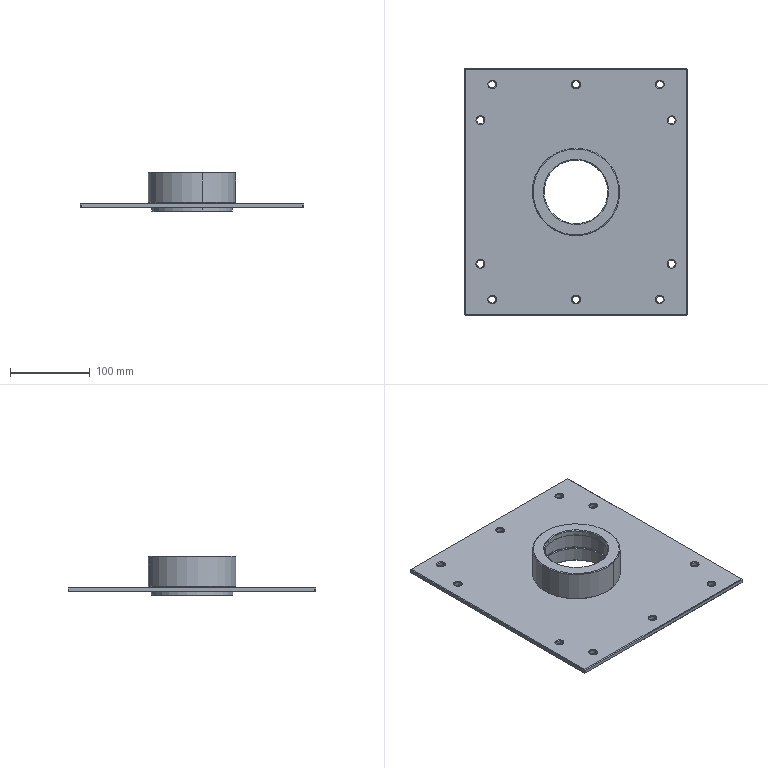Part | STEP file | 101000007789 | 2 solids | 125 faces | box 280 x 310 x 50 mm | volume 616529 mm3 | cone 62 | cylinder 34 | plane 29 | commonest cylinder face diameters 9 x20 90 x4 102 x4 80 x2 93.5 x2 110 x2